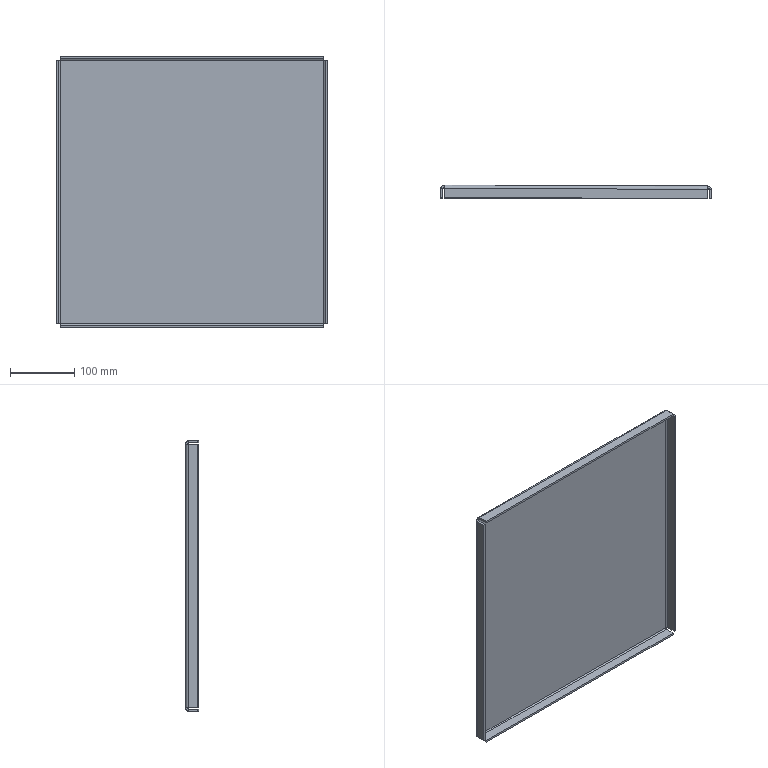Part | STEP file | Input 37 | 1 solid | 46 faces | box 420.785 x 20.607 x 420.745 mm | volume 642880 mm3 | plane 38 | cylinder 8 | commonest cylinder face diameters 4 x4 10.4 x4